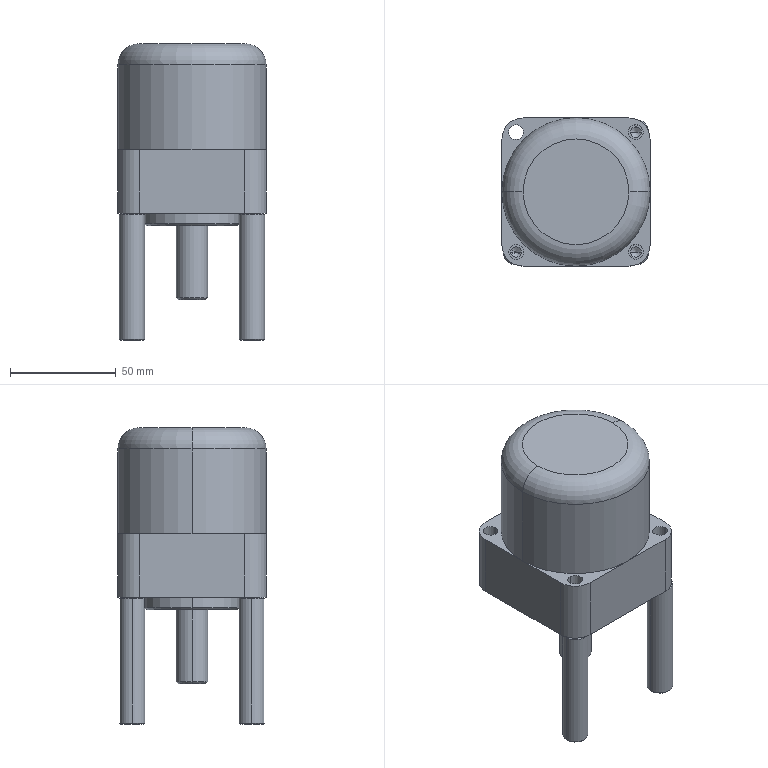Part | SolidWorks | features Chamfer 5, ICE 5, Fillet 2, HoleWzd 2, CirPattern 1, Extrusion 1 | 4 solids | 86 faces | box 70 x 70 x 140 mm | volume 361948 mm3 | cylinder 36 | cone 30 | plane 18 | torus 2 | commonest cylinder face diameters 5 x12 7 x8 12 x6 20 x4 15 x2 45 x2